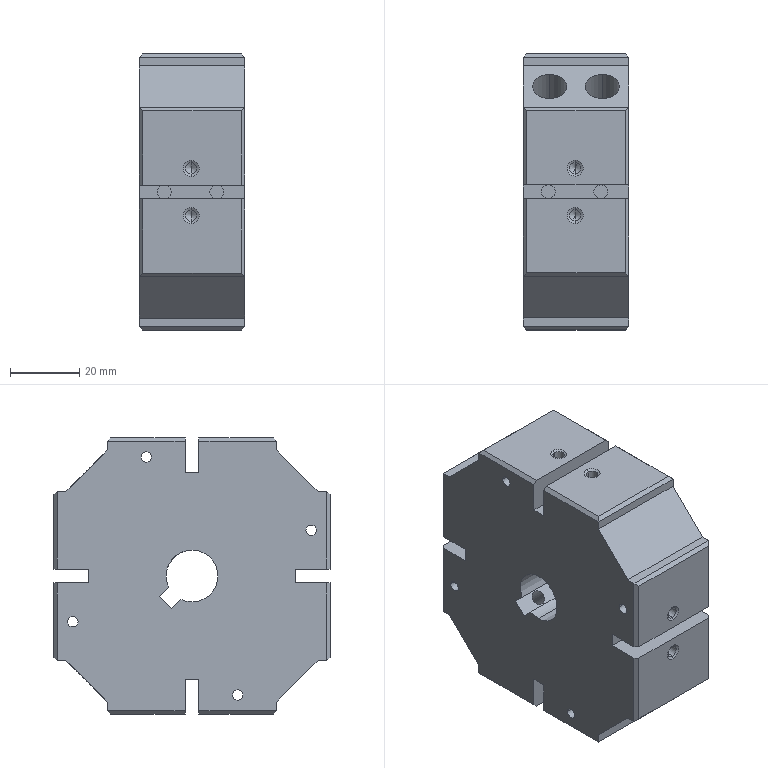Part | NX | 1 solid | 172 faces | box 30.5 x 80 x 80 mm | volume 156040 mm3 | plane 81 | cylinder 59 | cone 32 | commonest cylinder face diameters 3.3 x32 3 x8 4.2 x8 10 x8 15 x3